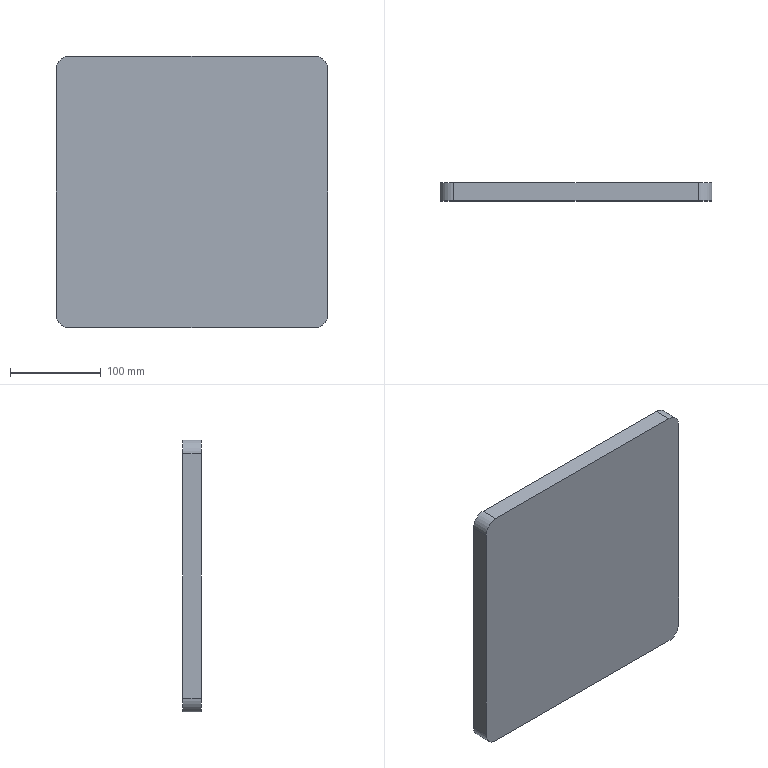Part | SolidWorks | features Extrusion 1 | 1 solid | 10 faces | box 300 x 20 x 300 mm | volume 1796137 mm3 | plane 6 | cylinder 4 | commonest cylinder face diameters 30 x4
STEP:
#1=CARTESIAN_POINT('',(-135.,0.,-150.));
#2=VERTEX_POINT('',#1);
#3=CARTESIAN_POINT('',(-150.,0.,-135.));
#4=VERTEX_POINT('',#3);
#5=CARTESIAN_POINT('',(-135.,0.,-135.));
#6=DIRECTION('',(0.,1.,0.));
#7=DIRECTION('',(0.,0.,1.));
#8=AXIS2_PLACEMENT_3D('',#5,#6,#7);
#9=CIRCLE('',#8,15.);
#10=EDGE_CURVE('',#2,#4,#9,.T.);
#11=ORIENTED_EDGE('',*,*,#10,.T.);
#12=CARTESIAN_POINT('',(-150.,20.,-135.));
#13=VERTEX_POINT('',#12);
#14=CARTESIAN_POINT('',(-150.,20.,-135.));
#15=DIRECTION('',(0.,-1.,0.));
#16=VECTOR('',#15,1000.);
#17=LINE('',#14,#16);
#18=EDGE_CURVE('',#13,#4,#17,.T.);
#19=ORIENTED_EDGE('',*,*,#18,.F.);
#20=CARTESIAN_POINT('',(-135.,20.,-150.));
#21=VERTEX_POINT('',#20);
#22=CARTESIAN_POINT('',(-135.,20.,-135.));
#23=DIRECTION('',(0.,1.,0.));
#24=DIRECTION('',(0.,0.,1.));
#25=AXIS2_PLACEMENT_3D('',#22,#23,#24);
#26=CIRCLE('',#25,15.);
#27=EDGE_CURVE('',#21,#13,#26,.T.);
#28=ORIENTED_EDGE('',*,*,#27,.F.);
#29=CARTESIAN_POINT('',(-135.,20.,-150.));
#30=DIRECTION('',(0.,-1.,0.));
#31=VECTOR('',#30,1000.);
#32=LINE('',#29,#31);
#33=EDGE_CURVE('',#21,#2,#32,.T.);
#34=ORIENTED_EDGE('',*,*,#33,.T.);
#35=EDGE_LOOP('',(#11,#19,#28,#34));
#36=FACE_OUTER_BOUND('',#35,.T.);
#37=CARTESIAN_POINT('',(-135.,20.,-135.));
#38=DIRECTION('',(0.,-1.,0.));
#39=DIRECTION('',(0.,0.,-1.));
#40=AXIS2_PLACEMENT_3D('',#37,#38,#39);
#41=CYLINDRICAL_SURFACE('',#40,15.);
#42=ADVANCED_FACE('',(#36),#41,.T.);
#43=CARTESIAN_POINT('',(-150.,0.,135.));
#44=VERTEX_POINT('',#43);
#45=CARTESIAN_POINT('',(-150.,0.,-135.));
#46=DIRECTION('',(0.,0.,1.));
#47=VECTOR('',#46,1000.);
#48=LINE('',#45,#47);
#49=EDGE_CURVE('',#4,#44,#48,.T.);
#50=ORIENTED_EDGE('',*,*,#49,.T.);
#51=CARTESIAN_POINT('',(-150.,20.,135.));
#52=VERTEX_POINT('',#51);
#53=CARTESIAN_POINT('',(-150.,20.,135.));
#54=DIRECTION('',(0.,-1.,0.));
#55=VECTOR('',#54,1000.);
#56=LINE('',#53,#55);
#57=EDGE_CURVE('',#52,#44,#56,.T.);
#58=ORIENTED_EDGE('',*,*,#57,.F.);
#59=CARTESIAN_POINT('',(-150.,20.,-135.));
#60=DIRECTION('',(0.,0.,1.));
#61=VECTOR('',#60,1000.);
#62=LINE('',#59,#61);
#63=EDGE_CURVE('',#13,#52,#62,.T.);
#64=ORIENTED_EDGE('',*,*,#63,.F.);
#65=ORIENTED_EDGE('',*,*,#18,.T.);
#66=EDGE_LOOP('',(#50,#58,#64,#65));
#67=FACE_OUTER_BOUND('',#66,.T.);
#68=CARTESIAN_POINT('',(-150.,20.,-135.));
#69=DIRECTION('',(1.,0.,0.));
#70=DIRECTION('',(0.,0.,-1.));
#71=AXIS2_PLACEMENT_3D('',#68,#69,#70);
#72=PLANE('',#71);
#73=ADVANCED_FACE('',(#67),#72,.F.);
#74=CARTESIAN_POINT('',(-135.,0.,150.));
#75=VERTEX_POINT('',#74);
#76=CARTESIAN_POINT('',(-135.,0.,135.));
#77=DIRECTION('',(0.,1.,0.));
#78=DIRECTION('',(0.,0.,-1.));
#79=AXIS2_PLACEMENT_3D('',#76,#77,#78);
#80=CIRCLE('',#79,15.);
#81=EDGE_CURVE('',#44,#75,#80,.T.);
#82=ORIENTED_EDGE('',*,*,#81,.T.);
#83=CARTESIAN_POINT('',(-135.,20.,150.));
#84=VERTEX_POINT('',#83);
#85=CARTESIAN_POINT('',(-135.,20.,150.));
#86=DIRECTION('',(0.,-1.,0.));
#87=VECTOR('',#86,1000.);
#88=LINE('',#85,#87);
#89=EDGE_CURVE('',#84,#75,#88,.T.);
#90=ORIENTED_EDGE('',*,*,#89,.F.);
#91=CARTESIAN_POINT('',(-135.,20.,135.));
#92=DIRECTION('',(0.,1.,0.));
#93=DIRECTION('',(0.,0.,-1.));
#94=AXIS2_PLACEMENT_3D('',#91,#92,#93);
#95=CIRCLE('',#94,15.);
#96=EDGE_CURVE('',#52,#84,#95,.T.);
#97=ORIENTED_EDGE('',*,*,#96,.F.);
#98=ORIENTED_EDGE('',*,*,#57,.T.);
#99=EDGE_LOOP('',(#82,#90,#97,#98));
#100=FACE_OUTER_BOUND('',#99,.T.);
#101=CARTESIAN_POINT('',(-135.,20.,135.));
#102=DIRECTION('',(0.,-1.,0.));
#103=DIRECTION('',(0.,0.,-1.));
#104=AXIS2_PLACEMENT_3D('',#101,#102,#103);
#105=CYLINDRICAL_SURFACE('',#104,15.);
#106=ADVANCED_FACE('',(#100),#105,.T.);
#107=CARTESIAN_POINT('',(135.,0.,150.));
#108=VERTEX_POINT('',#107);
#109=CARTESIAN_POINT('',(135.,0.,150.));
#110=DIRECTION('',(1.,0.,0.));
#111=VECTOR('',#110,1000.);
#112=LINE('',#109,#111);
#113=EDGE_CURVE('',#75,#108,#112,.T.);
#114=ORIENTED_EDGE('',*,*,#113,.T.);
#115=CARTESIAN_POINT('',(135.,20.,150.));
#116=VERTEX_POINT('',#115);
#117=CARTESIAN_POINT('',(135.,20.,150.));
#118=DIRECTION('',(0.,-1.,0.));
#119=VECTOR('',#118,1000.);
#120=LINE('',#117,#119);
#121=EDGE_CURVE('',#116,#108,#120,.T.);
#122=ORIENTED_EDGE('',*,*,#121,.F.);
#123=CARTESIAN_POINT('',(135.,20.,150.));
#124=DIRECTION('',(1.,0.,0.));
#125=VECTOR('',#124,1000.);
#126=LINE('',#123,#125);
#127=EDGE_CURVE('',#84,#116,#126,.T.);
#128=ORIENTED_EDGE('',*,*,#127,.F.);
#129=ORIENTED_EDGE('',*,*,#89,.T.);
#130=EDGE_LOOP('',(#114,#122,#128,#129));
#131=FACE_OUTER_BOUND('',#130,.T.);
#132=CARTESIAN_POINT('',(135.,20.,150.));
#133=DIRECTION('',(0.,0.,-1.));
#134=DIRECTION('',(-1.,0.,0.));
#135=AXIS2_PLACEMENT_3D('',#132,#133,#134);
#136=PLANE('',#135);
#137=ADVANCED_FACE('',(#131),#136,.F.);
#138=CARTESIAN_POINT('',(150.,0.,135.));
#139=VERTEX_POINT('',#138);
#140=CARTESIAN_POINT('',(135.,0.,135.));
#141=DIRECTION('',(0.,1.,0.));
#142=DIRECTION('',(0.,0.,1.));
#143=AXIS2_PLACEMENT_3D('',#140,#141,#142);
#144=CIRCLE('',#143,15.);
#145=EDGE_CURVE('',#108,#139,#144,.T.);
#146=ORIENTED_EDGE('',*,*,#145,.T.);
#147=CARTESIAN_POINT('',(150.,20.,135.));
#148=VERTEX_POINT('',#147);
#149=CARTESIAN_POINT('',(150.,20.,135.));
#150=DIRECTION('',(0.,-1.,0.));
#151=VECTOR('',#150,1000.);
#152=LINE('',#149,#151);
#153=EDGE_CURVE('',#148,#139,#152,.T.);
#154=ORIENTED_EDGE('',*,*,#153,.F.);
#155=CARTESIAN_POINT('',(135.,20.,135.));
#156=DIRECTION('',(0.,1.,0.));
#157=DIRECTION('',(0.,0.,1.));
#158=AXIS2_PLACEMENT_3D('',#155,#156,#157);
#159=CIRCLE('',#158,15.);
#160=EDGE_CURVE('',#116,#148,#159,.T.);
#161=ORIENTED_EDGE('',*,*,#160,.F.);
#162=ORIENTED_EDGE('',*,*,#121,.T.);
#163=EDGE_LOOP('',(#146,#154,#161,#162));
#164=FACE_OUTER_BOUND('',#163,.T.);
#165=CARTESIAN_POINT('',(135.,20.,135.));
#166=DIRECTION('',(0.,-1.,0.));
#167=DIRECTION('',(0.,0.,-1.));
#168=AXIS2_PLACEMENT_3D('',#165,#166,#167);
#169=CYLINDRICAL_SURFACE('',#168,15.);
#170=ADVANCED_FACE('',(#164),#169,.T.);
#171=CARTESIAN_POINT('',(150.,0.,-135.));
#172=VERTEX_POINT('',#171);
#173=CARTESIAN_POINT('',(150.,0.,-135.));
#174=DIRECTION('',(0.,0.,-1.));
#175=VECTOR('',#174,1000.);
#176=LINE('',#173,#175);
#177=EDGE_CURVE('',#139,#172,#176,.T.);
#178=ORIENTED_EDGE('',*,*,#177,.T.);
#179=CARTESIAN_POINT('',(150.,20.,-135.));
#180=VERTEX_POINT('',#179);
#181=CARTESIAN_POINT('',(150.,20.,-135.));
#182=DIRECTION('',(0.,-1.,0.));
#183=VECTOR('',#182,1000.);
#184=LINE('',#181,#183);
#185=EDGE_CURVE('',#180,#172,#184,.T.);
#186=ORIENTED_EDGE('',*,*,#185,.F.);
#187=CARTESIAN_POINT('',(150.,20.,-135.));
#188=DIRECTION('',(0.,0.,-1.));
#189=VECTOR('',#188,1000.);
#190=LINE('',#187,#189);
#191=EDGE_CURVE('',#148,#180,#190,.T.);
#192=ORIENTED_EDGE('',*,*,#191,.F.);
#193=ORIENTED_EDGE('',*,*,#153,.T.);
#194=EDGE_LOOP('',(#178,#186,#192,#193));
#195=FACE_OUTER_BOUND('',#194,.T.);
#196=CARTESIAN_POINT('',(150.,20.,-135.));
#197=DIRECTION('',(-1.,0.,0.));
#198=DIRECTION('',(0.,0.,1.));
#199=AXIS2_PLACEMENT_3D('',#196,#197,#198);
#200=PLANE('',#199);
#201=ADVANCED_FACE('',(#195),#200,.F.);
#202=CARTESIAN_POINT('',(135.,0.,-150.));
#203=VERTEX_POINT('',#202);
#204=CARTESIAN_POINT('',(135.,0.,-135.));
#205=DIRECTION('',(0.,1.,0.));
#206=DIRECTION('',(0.,0.,-1.));
#207=AXIS2_PLACEMENT_3D('',#204,#205,#206);
#208=CIRCLE('',#207,15.);
#209=EDGE_CURVE('',#172,#203,#208,.T.);
#210=ORIENTED_EDGE('',*,*,#209,.T.);
#211=CARTESIAN_POINT('',(135.,20.,-150.));
#212=VERTEX_POINT('',#211);
#213=CARTESIAN_POINT('',(135.,20.,-150.));
#214=DIRECTION('',(0.,-1.,0.));
#215=VECTOR('',#214,1000.);
#216=LINE('',#213,#215);
#217=EDGE_CURVE('',#212,#203,#216,.T.);
#218=ORIENTED_EDGE('',*,*,#217,.F.);
#219=CARTESIAN_POINT('',(135.,20.,-135.));
#220=DIRECTION('',(0.,1.,0.));
#221=DIRECTION('',(0.,0.,-1.));
#222=AXIS2_PLACEMENT_3D('',#219,#220,#221);
#223=CIRCLE('',#222,15.);
#224=EDGE_CURVE('',#180,#212,#223,.T.);
#225=ORIENTED_EDGE('',*,*,#224,.F.);
#226=ORIENTED_EDGE('',*,*,#185,.T.);
#227=EDGE_LOOP('',(#210,#218,#225,#226));
#228=FACE_OUTER_BOUND('',#227,.T.);
#229=CARTESIAN_POINT('',(135.,20.,-135.));
#230=DIRECTION('',(0.,-1.,0.));
#231=DIRECTION('',(0.,0.,-1.));
#232=AXIS2_PLACEMENT_3D('',#229,#230,#231);
#233=CYLINDRICAL_SURFACE('',#232,15.);
#234=ADVANCED_FACE('',(#228),#233,.T.);
#235=CARTESIAN_POINT('',(135.,0.,-150.));
#236=DIRECTION('',(-1.,0.,0.));
#237=VECTOR('',#236,1000.);
#238=LINE('',#235,#237);
#239=EDGE_CURVE('',#203,#2,#238,.T.);
#240=ORIENTED_EDGE('',*,*,#239,.T.);
#241=ORIENTED_EDGE('',*,*,#33,.F.);
#242=CARTESIAN_POINT('',(135.,20.,-150.));
#243=DIRECTION('',(-1.,0.,0.));
#244=VECTOR('',#243,1000.);
#245=LINE('',#242,#244);
#246=EDGE_CURVE('',#212,#21,#245,.T.);
#247=ORIENTED_EDGE('',*,*,#246,.F.);
#248=ORIENTED_EDGE('',*,*,#217,.T.);
#249=EDGE_LOOP('',(#240,#241,#247,#248));
#250=FACE_OUTER_BOUND('',#249,.T.);
#251=CARTESIAN_POINT('',(135.,20.,-150.));
#252=DIRECTION('',(0.,0.,1.));
#253=DIRECTION('',(1.,0.,0.));
#254=AXIS2_PLACEMENT_3D('',#251,#252,#253);
#255=PLANE('',#254);
#256=ADVANCED_FACE('',(#250),#255,.F.);
#257=ORIENTED_EDGE('',*,*,#27,.T.);
#258=ORIENTED_EDGE('',*,*,#63,.T.);
#259=ORIENTED_EDGE('',*,*,#96,.T.);
#260=ORIENTED_EDGE('',*,*,#127,.T.);
#261=ORIENTED_EDGE('',*,*,#160,.T.);
#262=ORIENTED_EDGE('',*,*,#191,.T.);
#263=ORIENTED_EDGE('',*,*,#224,.T.);
#264=ORIENTED_EDGE('',*,*,#246,.T.);
#265=EDGE_LOOP('',(#257,#258,#259,#260,#261,#262,#263,#264));
#266=FACE_OUTER_BOUND('',#265,.T.);
#267=CARTESIAN_POINT('',(-135.,20.,-135.));
#268=DIRECTION('',(0.,1.,0.));
#269=DIRECTION('',(0.,0.,1.));
#270=AXIS2_PLACEMENT_3D('',#267,#268,#269);
#271=PLANE('',#270);
#272=ADVANCED_FACE('',(#266),#271,.T.);
#273=ORIENTED_EDGE('',*,*,#10,.F.);
#274=ORIENTED_EDGE('',*,*,#239,.F.);
#275=ORIENTED_EDGE('',*,*,#209,.F.);
#276=ORIENTED_EDGE('',*,*,#177,.F.);
#277=ORIENTED_EDGE('',*,*,#145,.F.);
#278=ORIENTED_EDGE('',*,*,#113,.F.);
#279=ORIENTED_EDGE('',*,*,#81,.F.);
#280=ORIENTED_EDGE('',*,*,#49,.F.);
#281=EDGE_LOOP('',(#273,#274,#275,#276,#277,#278,#279,#280));
#282=FACE_OUTER_BOUND('',#281,.T.);
#283=CARTESIAN_POINT('',(-135.,0.,-135.));
#284=DIRECTION('',(0.,1.,0.));
#285=DIRECTION('',(0.,0.,1.));
#286=AXIS2_PLACEMENT_3D('',#283,#284,#285);
#287=PLANE('',#286);
#288=ADVANCED_FACE('',(#282),#287,.F.);
#289=CLOSED_SHELL('',(#42,#73,#106,#137,#170,#201,#234,#256,#272,#288));
#290=MANIFOLD_SOLID_BREP('',#289);
#291=CARTESIAN_POINT('',(0.,0.,0.));
#292=DIRECTION('',(0.,0.,1.));
#293=DIRECTION('',(1.,0.,0.));
#294=AXIS2_PLACEMENT_3D('',#291,#292,#293);
#295=(LENGTH_UNIT()NAMED_UNIT(*)SI_UNIT(.MILLI.,.METRE.));
#296=UNCERTAINTY_MEASURE_WITH_UNIT(LENGTH_MEASURE(0.00001),#295,'','');
#297=(NAMED_UNIT(*)PLANE_ANGLE_UNIT()SI_UNIT($,.RADIAN.));
#298=(NAMED_UNIT(*)SI_UNIT($,.STERADIAN.)SOLID_ANGLE_UNIT());
#299=(GEOMETRIC_REPRESENTATION_CONTEXT(3)GLOBAL_UNCERTAINTY_ASSIGNED_CONTEXT((#296))GLOBAL_UNIT_ASSIGNED_CONTEXT((#295,#297,#298))REPRESENTATION_CONTEXT('',''));
#300=ADVANCED_BREP_SHAPE_REPRESENTATION('',(#290,#294),#299);